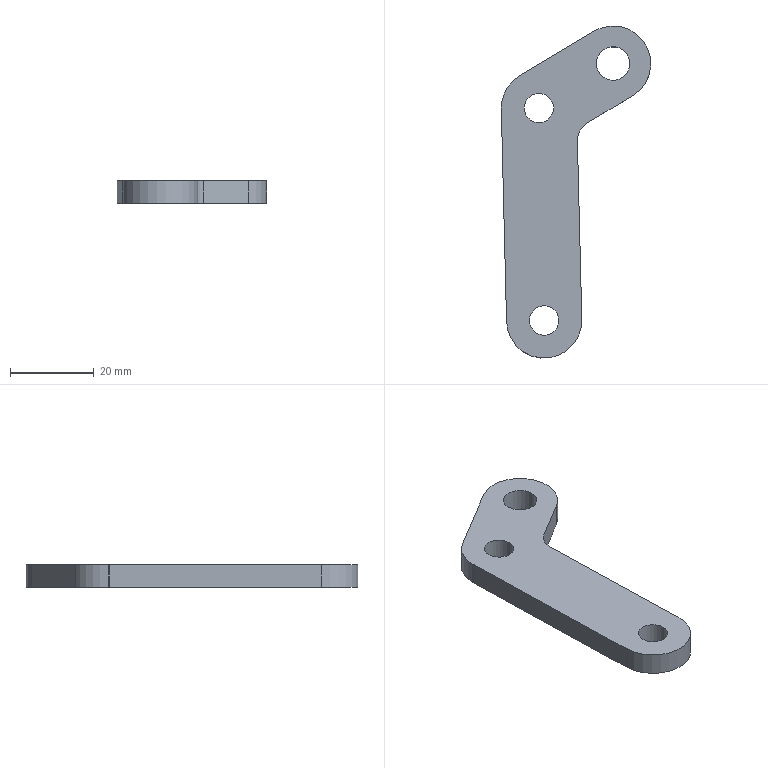Part | SolidWorks | features Extrusion 1 | 1 solid | 18 faces | box 35.738 x 79.423 x 5.4 mm | volume 7618 mm3 | cylinder 12 | plane 6 | commonest cylinder face diameters 7 x4 18 x3 8 x2 10.009 x2 17.997 x1
STEP:
#1=CARTESIAN_POINT('',(11.627,34.256,5.4));
#2=VERTEX_POINT('',#1);
#3=CARTESIAN_POINT('',(9.196,29.964,5.4));
#4=VERTEX_POINT('',#3);
#5=CARTESIAN_POINT('',(14.201,29.964,5.4));
#6=DIRECTION('',(0.,0.,1.));
#7=DIRECTION('',(1.,0.,0.));
#8=AXIS2_PLACEMENT_3D('',#5,#6,#7);
#9=CIRCLE('',#8,5.004);
#10=EDGE_CURVE('',#2,#4,#9,.T.);
#11=ORIENTED_EDGE('',*,*,#10,.T.);
#12=CARTESIAN_POINT('',(9.196,29.964,0.));
#13=VERTEX_POINT('',#12);
#14=CARTESIAN_POINT('',(9.196,29.964,5.4));
#15=DIRECTION('',(0.,0.,-1.));
#16=VECTOR('',#15,1000.);
#17=LINE('',#14,#16);
#18=EDGE_CURVE('',#4,#13,#17,.T.);
#19=ORIENTED_EDGE('',*,*,#18,.T.);
#20=CARTESIAN_POINT('',(11.627,34.256,0.));
#21=VERTEX_POINT('',#20);
#22=CARTESIAN_POINT('',(14.201,29.964,0.));
#23=DIRECTION('',(0.,0.,1.));
#24=DIRECTION('',(1.,0.,0.));
#25=AXIS2_PLACEMENT_3D('',#22,#23,#24);
#26=CIRCLE('',#25,5.004);
#27=EDGE_CURVE('',#21,#13,#26,.T.);
#28=ORIENTED_EDGE('',*,*,#27,.F.);
#29=CARTESIAN_POINT('',(11.627,34.256,5.4));
#30=DIRECTION('',(0.,0.,-1.));
#31=VECTOR('',#30,1000.);
#32=LINE('',#29,#31);
#33=EDGE_CURVE('',#2,#21,#32,.T.);
#34=ORIENTED_EDGE('',*,*,#33,.F.);
#35=EDGE_LOOP('',(#11,#19,#28,#34));
#36=FACE_OUTER_BOUND('',#35,.T.);
#37=CARTESIAN_POINT('',(14.201,29.964,5.4));
#38=DIRECTION('',(0.,0.,-1.));
#39=DIRECTION('',(-1.,0.,0.));
#40=AXIS2_PLACEMENT_3D('',#37,#38,#39);
#41=CYLINDRICAL_SURFACE('',#40,5.004);
#42=ADVANCED_FACE('',(#36),#41,.F.);
#43=CARTESIAN_POINT('',(-3.5,37.774,5.4));
#44=VERTEX_POINT('',#43);
#45=CARTESIAN_POINT('',(3.5,37.774,5.4));
#46=VERTEX_POINT('',#45);
#47=CARTESIAN_POINT('',(0.,37.774,5.4));
#48=DIRECTION('',(0.,0.,1.));
#49=DIRECTION('',(1.,0.,0.));
#50=AXIS2_PLACEMENT_3D('',#47,#48,#49);
#51=CIRCLE('',#50,3.5);
#52=EDGE_CURVE('',#44,#46,#51,.T.);
#53=ORIENTED_EDGE('',*,*,#52,.T.);
#54=CARTESIAN_POINT('',(3.5,37.774,0.));
#55=VERTEX_POINT('',#54);
#56=CARTESIAN_POINT('',(3.5,37.774,5.4));
#57=DIRECTION('',(0.,0.,-1.));
#58=VECTOR('',#57,1000.);
#59=LINE('',#56,#58);
#60=EDGE_CURVE('',#46,#55,#59,.T.);
#61=ORIENTED_EDGE('',*,*,#60,.T.);
#62=CARTESIAN_POINT('',(-3.5,37.774,0.));
#63=VERTEX_POINT('',#62);
#64=CARTESIAN_POINT('',(0.,37.774,0.));
#65=DIRECTION('',(0.,0.,1.));
#66=DIRECTION('',(1.,0.,0.));
#67=AXIS2_PLACEMENT_3D('',#64,#65,#66);
#68=CIRCLE('',#67,3.5);
#69=EDGE_CURVE('',#63,#55,#68,.T.);
#70=ORIENTED_EDGE('',*,*,#69,.F.);
#71=CARTESIAN_POINT('',(-3.5,37.774,5.4));
#72=DIRECTION('',(0.,0.,-1.));
#73=VECTOR('',#72,1000.);
#74=LINE('',#71,#73);
#75=EDGE_CURVE('',#44,#63,#74,.T.);
#76=ORIENTED_EDGE('',*,*,#75,.F.);
#77=EDGE_LOOP('',(#53,#61,#70,#76));
#78=FACE_OUTER_BOUND('',#77,.T.);
#79=CARTESIAN_POINT('',(0.,37.774,5.4));
#80=DIRECTION('',(0.,0.,-1.));
#81=DIRECTION('',(-1.,0.,0.));
#82=AXIS2_PLACEMENT_3D('',#79,#80,#81);
#83=CYLINDRICAL_SURFACE('',#82,3.5);
#84=ADVANCED_FACE('',(#78),#83,.F.);
#85=CARTESIAN_POINT('',(-2.25,-13.01,5.4));
#86=VERTEX_POINT('',#85);
#87=CARTESIAN_POINT('',(4.75,-13.01,5.4));
#88=VERTEX_POINT('',#87);
#89=CARTESIAN_POINT('',(1.25,-13.01,5.4));
#90=DIRECTION('',(0.,0.,1.));
#91=DIRECTION('',(1.,0.,0.));
#92=AXIS2_PLACEMENT_3D('',#89,#90,#91);
#93=CIRCLE('',#92,3.5);
#94=EDGE_CURVE('',#86,#88,#93,.T.);
#95=ORIENTED_EDGE('',*,*,#94,.T.);
#96=CARTESIAN_POINT('',(4.75,-13.01,0.));
#97=VERTEX_POINT('',#96);
#98=CARTESIAN_POINT('',(4.75,-13.01,5.4));
#99=DIRECTION('',(0.,0.,-1.));
#100=VECTOR('',#99,1000.);
#101=LINE('',#98,#100);
#102=EDGE_CURVE('',#88,#97,#101,.T.);
#103=ORIENTED_EDGE('',*,*,#102,.T.);
#104=CARTESIAN_POINT('',(-2.25,-13.01,0.));
#105=VERTEX_POINT('',#104);
#106=CARTESIAN_POINT('',(1.25,-13.01,0.));
#107=DIRECTION('',(0.,0.,1.));
#108=DIRECTION('',(1.,0.,0.));
#109=AXIS2_PLACEMENT_3D('',#106,#107,#108);
#110=CIRCLE('',#109,3.5);
#111=EDGE_CURVE('',#105,#97,#110,.T.);
#112=ORIENTED_EDGE('',*,*,#111,.F.);
#113=CARTESIAN_POINT('',(-2.25,-13.01,5.4));
#114=DIRECTION('',(0.,0.,-1.));
#115=VECTOR('',#114,1000.);
#116=LINE('',#113,#115);
#117=EDGE_CURVE('',#86,#105,#116,.T.);
#118=ORIENTED_EDGE('',*,*,#117,.F.);
#119=EDGE_LOOP('',(#95,#103,#112,#118));
#120=FACE_OUTER_BOUND('',#119,.T.);
#121=CARTESIAN_POINT('',(1.25,-13.01,5.4));
#122=DIRECTION('',(0.,0.,-1.));
#123=DIRECTION('',(-1.,0.,0.));
#124=AXIS2_PLACEMENT_3D('',#121,#122,#123);
#125=CYLINDRICAL_SURFACE('',#124,3.5);
#126=ADVANCED_FACE('',(#120),#125,.F.);
#127=CARTESIAN_POINT('',(13.74,48.414,5.4));
#128=VERTEX_POINT('',#127);
#129=CARTESIAN_POINT('',(21.74,48.414,5.4));
#130=VERTEX_POINT('',#129);
#131=CARTESIAN_POINT('',(17.74,48.414,5.4));
#132=DIRECTION('',(0.,0.,1.));
#133=DIRECTION('',(1.,0.,0.));
#134=AXIS2_PLACEMENT_3D('',#131,#132,#133);
#135=CIRCLE('',#134,4.);
#136=EDGE_CURVE('',#128,#130,#135,.T.);
#137=ORIENTED_EDGE('',*,*,#136,.T.);
#138=CARTESIAN_POINT('',(21.74,48.414,0.));
#139=VERTEX_POINT('',#138);
#140=CARTESIAN_POINT('',(21.74,48.414,5.4));
#141=DIRECTION('',(0.,0.,-1.));
#142=VECTOR('',#141,1000.);
#143=LINE('',#140,#142);
#144=EDGE_CURVE('',#130,#139,#143,.T.);
#145=ORIENTED_EDGE('',*,*,#144,.T.);
#146=CARTESIAN_POINT('',(13.74,48.414,0.));
#147=VERTEX_POINT('',#146);
#148=CARTESIAN_POINT('',(17.74,48.414,0.));
#149=DIRECTION('',(0.,0.,1.));
#150=DIRECTION('',(1.,0.,0.));
#151=AXIS2_PLACEMENT_3D('',#148,#149,#150);
#152=CIRCLE('',#151,4.);
#153=EDGE_CURVE('',#147,#139,#152,.T.);
#154=ORIENTED_EDGE('',*,*,#153,.F.);
#155=CARTESIAN_POINT('',(13.74,48.414,5.4));
#156=DIRECTION('',(0.,0.,-1.));
#157=VECTOR('',#156,1000.);
#158=LINE('',#155,#157);
#159=EDGE_CURVE('',#128,#147,#158,.T.);
#160=ORIENTED_EDGE('',*,*,#159,.F.);
#161=EDGE_LOOP('',(#137,#145,#154,#160));
#162=FACE_OUTER_BOUND('',#161,.T.);
#163=CARTESIAN_POINT('',(17.74,48.414,5.4));
#164=DIRECTION('',(0.,0.,-1.));
#165=DIRECTION('',(-1.,0.,0.));
#166=AXIS2_PLACEMENT_3D('',#163,#164,#165);
#167=CYLINDRICAL_SURFACE('',#166,4.);
#168=ADVANCED_FACE('',(#162),#167,.F.);
#169=CARTESIAN_POINT('',(-9.,37.774,5.4));
#170=VERTEX_POINT('',#169);
#171=CARTESIAN_POINT('',(-8.997,37.553,5.4));
#172=VERTEX_POINT('',#171);
#173=CARTESIAN_POINT('',(0.,37.774,5.4));
#174=DIRECTION('',(0.,0.,1.));
#175=DIRECTION('',(1.,0.,0.));
#176=AXIS2_PLACEMENT_3D('',#173,#174,#175);
#177=CIRCLE('',#176,9.);
#178=EDGE_CURVE('',#170,#172,#177,.T.);
#179=ORIENTED_EDGE('',*,*,#178,.F.);
#180=CARTESIAN_POINT('',(-9.,37.774,0.));
#181=VERTEX_POINT('',#180);
#182=CARTESIAN_POINT('',(-9.,37.774,5.4));
#183=DIRECTION('',(0.,0.,-1.));
#184=VECTOR('',#183,1000.);
#185=LINE('',#182,#184);
#186=EDGE_CURVE('',#170,#181,#185,.T.);
#187=ORIENTED_EDGE('',*,*,#186,.T.);
#188=CARTESIAN_POINT('',(-8.997,37.553,0.));
#189=VERTEX_POINT('',#188);
#190=CARTESIAN_POINT('',(0.,37.774,0.));
#191=DIRECTION('',(0.,0.,1.));
#192=DIRECTION('',(1.,0.,0.));
#193=AXIS2_PLACEMENT_3D('',#190,#191,#192);
#194=CIRCLE('',#193,9.);
#195=EDGE_CURVE('',#181,#189,#194,.T.);
#196=ORIENTED_EDGE('',*,*,#195,.T.);
#197=CARTESIAN_POINT('',(-8.997,37.553,5.4));
#198=DIRECTION('',(0.,0.,-1.));
#199=VECTOR('',#198,1000.);
#200=LINE('',#197,#199);
#201=EDGE_CURVE('',#172,#189,#200,.T.);
#202=ORIENTED_EDGE('',*,*,#201,.F.);
#203=EDGE_LOOP('',(#179,#187,#196,#202));
#204=FACE_OUTER_BOUND('',#203,.T.);
#205=CARTESIAN_POINT('',(0.,37.774,5.4));
#206=DIRECTION('',(0.,0.,-1.));
#207=DIRECTION('',(-1.,0.,0.));
#208=AXIS2_PLACEMENT_3D('',#205,#206,#207);
#209=CYLINDRICAL_SURFACE('',#208,9.);
#210=ADVANCED_FACE('',(#204),#209,.T.);
#211=CARTESIAN_POINT('',(22.368,40.697,0.));
#212=VERTEX_POINT('',#211);
#213=CARTESIAN_POINT('',(-12.034,20.067,0.));
#214=DIRECTION('',(-0.8576,-0.5143,0.));
#215=VECTOR('',#214,1000.);
#216=LINE('',#213,#215);
#217=EDGE_CURVE('',#212,#21,#216,.T.);
#218=ORIENTED_EDGE('',*,*,#217,.F.);
#219=CARTESIAN_POINT('',(22.368,40.697,5.4));
#220=VERTEX_POINT('',#219);
#221=CARTESIAN_POINT('',(22.368,40.697,5.4));
#222=DIRECTION('',(0.,0.,-1.));
#223=VECTOR('',#222,1000.);
#224=LINE('',#221,#223);
#225=EDGE_CURVE('',#220,#212,#224,.T.);
#226=ORIENTED_EDGE('',*,*,#225,.F.);
#227=CARTESIAN_POINT('',(-12.034,20.067,5.4));
#228=DIRECTION('',(-0.8576,-0.5143,0.));
#229=VECTOR('',#228,1000.);
#230=LINE('',#227,#229);
#231=EDGE_CURVE('',#220,#2,#230,.T.);
#232=ORIENTED_EDGE('',*,*,#231,.T.);
#233=ORIENTED_EDGE('',*,*,#33,.T.);
#234=EDGE_LOOP('',(#218,#226,#232,#233));
#235=FACE_OUTER_BOUND('',#234,.T.);
#236=CARTESIAN_POINT('',(-12.034,20.067,5.4));
#237=DIRECTION('',(0.5143,-0.8576,0.));
#238=DIRECTION('',(0.8576,0.5143,0.));
#239=AXIS2_PLACEMENT_3D('',#236,#237,#238);
#240=PLANE('',#239);
#241=ADVANCED_FACE('',(#235),#240,.T.);
#242=CARTESIAN_POINT('',(13.112,56.132,0.));
#243=VERTEX_POINT('',#242);
#244=CARTESIAN_POINT('',(17.74,48.414,0.));
#245=DIRECTION('',(0.,0.,1.));
#246=DIRECTION('',(1.,0.,0.));
#247=AXIS2_PLACEMENT_3D('',#244,#245,#246);
#248=CIRCLE('',#247,8.998);
#249=EDGE_CURVE('',#212,#243,#248,.T.);
#250=ORIENTED_EDGE('',*,*,#249,.T.);
#251=CARTESIAN_POINT('',(13.112,56.132,5.4));
#252=VERTEX_POINT('',#251);
#253=CARTESIAN_POINT('',(13.112,56.132,5.4));
#254=DIRECTION('',(0.,0.,-1.));
#255=VECTOR('',#254,1000.);
#256=LINE('',#253,#255);
#257=EDGE_CURVE('',#252,#243,#256,.T.);
#258=ORIENTED_EDGE('',*,*,#257,.F.);
#259=CARTESIAN_POINT('',(17.74,48.414,5.4));
#260=DIRECTION('',(0.,0.,1.));
#261=DIRECTION('',(1.,0.,0.));
#262=AXIS2_PLACEMENT_3D('',#259,#260,#261);
#263=CIRCLE('',#262,8.998);
#264=EDGE_CURVE('',#220,#252,#263,.T.);
#265=ORIENTED_EDGE('',*,*,#264,.F.);
#266=ORIENTED_EDGE('',*,*,#225,.T.);
#267=EDGE_LOOP('',(#250,#258,#265,#266));
#268=FACE_OUTER_BOUND('',#267,.T.);
#269=CARTESIAN_POINT('',(17.74,48.414,5.4));
#270=DIRECTION('',(0.,0.,-1.));
#271=DIRECTION('',(-1.,0.,0.));
#272=AXIS2_PLACEMENT_3D('',#269,#270,#271);
#273=CYLINDRICAL_SURFACE('',#272,8.998);
#274=ADVANCED_FACE('',(#268),#273,.T.);
#275=CARTESIAN_POINT('',(-4.629,45.493,0.));
#276=VERTEX_POINT('',#275);
#277=CARTESIAN_POINT('',(-21.289,35.502,0.));
#278=DIRECTION('',(0.8576,0.5143,0.));
#279=VECTOR('',#278,1000.);
#280=LINE('',#277,#279);
#281=EDGE_CURVE('',#276,#243,#280,.T.);
#282=ORIENTED_EDGE('',*,*,#281,.F.);
#283=CARTESIAN_POINT('',(-4.629,45.493,5.4));
#284=VERTEX_POINT('',#283);
#285=CARTESIAN_POINT('',(-4.629,45.493,5.4));
#286=DIRECTION('',(0.,0.,-1.));
#287=VECTOR('',#286,1000.);
#288=LINE('',#285,#287);
#289=EDGE_CURVE('',#284,#276,#288,.T.);
#290=ORIENTED_EDGE('',*,*,#289,.F.);
#291=CARTESIAN_POINT('',(-21.289,35.502,5.4));
#292=DIRECTION('',(0.8576,0.5143,0.));
#293=VECTOR('',#292,1000.);
#294=LINE('',#291,#293);
#295=EDGE_CURVE('',#284,#252,#294,.T.);
#296=ORIENTED_EDGE('',*,*,#295,.T.);
#297=ORIENTED_EDGE('',*,*,#257,.T.);
#298=EDGE_LOOP('',(#282,#290,#296,#297));
#299=FACE_OUTER_BOUND('',#298,.T.);
#300=CARTESIAN_POINT('',(-21.289,35.502,5.4));
#301=DIRECTION('',(-0.5143,0.8576,0.));
#302=DIRECTION('',(-0.8576,-0.5143,0.));
#303=AXIS2_PLACEMENT_3D('',#300,#301,#302);
#304=PLANE('',#303);
#305=ADVANCED_FACE('',(#299),#304,.T.);
#306=ORIENTED_EDGE('',*,*,#186,.F.);
#307=CARTESIAN_POINT('',(0.,37.774,5.4));
#308=DIRECTION('',(0.,0.,1.));
#309=DIRECTION('',(1.,0.,0.));
#310=AXIS2_PLACEMENT_3D('',#307,#308,#309);
#311=CIRCLE('',#310,9.);
#312=EDGE_CURVE('',#284,#170,#311,.T.);
#313=ORIENTED_EDGE('',*,*,#312,.F.);
#314=ORIENTED_EDGE('',*,*,#289,.T.);
#315=CARTESIAN_POINT('',(0.,37.774,0.));
#316=DIRECTION('',(0.,0.,1.));
#317=DIRECTION('',(1.,0.,0.));
#318=AXIS2_PLACEMENT_3D('',#315,#316,#317);
#319=CIRCLE('',#318,9.);
#320=EDGE_CURVE('',#276,#181,#319,.T.);
#321=ORIENTED_EDGE('',*,*,#320,.T.);
#322=EDGE_LOOP('',(#306,#313,#314,#321));
#323=FACE_OUTER_BOUND('',#322,.T.);
#324=CARTESIAN_POINT('',(0.,37.774,5.4));
#325=DIRECTION('',(0.,0.,-1.));
#326=DIRECTION('',(-1.,0.,0.));
#327=AXIS2_PLACEMENT_3D('',#324,#325,#326);
#328=CYLINDRICAL_SURFACE('',#327,9.);
#329=ADVANCED_FACE('',(#323),#328,.T.);
#330=CARTESIAN_POINT('',(-7.747,-13.232,0.));
#331=VERTEX_POINT('',#330);
#332=CARTESIAN_POINT('',(-8.068,-0.1986,0.));
#333=DIRECTION('',(0.02461,-0.9997,0.));
#334=VECTOR('',#333,1000.);
#335=LINE('',#332,#334);
#336=EDGE_CURVE('',#189,#331,#335,.T.);
#337=ORIENTED_EDGE('',*,*,#336,.T.);
#338=CARTESIAN_POINT('',(-7.747,-13.232,5.4));
#339=VERTEX_POINT('',#338);
#340=CARTESIAN_POINT('',(-7.747,-13.232,5.4));
#341=DIRECTION('',(0.,0.,-1.));
#342=VECTOR('',#341,1000.);
#343=LINE('',#340,#342);
#344=EDGE_CURVE('',#339,#331,#343,.T.);
#345=ORIENTED_EDGE('',*,*,#344,.F.);
#346=CARTESIAN_POINT('',(-8.068,-0.1986,5.4));
#347=DIRECTION('',(0.02461,-0.9997,0.));
#348=VECTOR('',#347,1000.);
#349=LINE('',#346,#348);
#350=EDGE_CURVE('',#172,#339,#349,.T.);
#351=ORIENTED_EDGE('',*,*,#350,.F.);
#352=ORIENTED_EDGE('',*,*,#201,.T.);
#353=EDGE_LOOP('',(#337,#345,#351,#352));
#354=FACE_OUTER_BOUND('',#353,.T.);
#355=CARTESIAN_POINT('',(-8.068,-0.1986,5.4));
#356=DIRECTION('',(0.9997,0.02461,0.));
#357=DIRECTION('',(-0.02461,0.9997,0.));
#358=AXIS2_PLACEMENT_3D('',#355,#356,#357);
#359=PLANE('',#358);
#360=ADVANCED_FACE('',(#354),#359,.F.);
#361=CARTESIAN_POINT('',(10.247,-12.789,0.));
#362=VERTEX_POINT('',#361);
#363=CARTESIAN_POINT('',(1.25,-13.01,0.));
#364=DIRECTION('',(0.,0.,1.));
#365=DIRECTION('',(1.,0.,0.));
#366=AXIS2_PLACEMENT_3D('',#363,#364,#365);
#367=CIRCLE('',#366,9.);
#368=EDGE_CURVE('',#331,#362,#367,.T.);
#369=ORIENTED_EDGE('',*,*,#368,.T.);
#370=CARTESIAN_POINT('',(10.247,-12.789,5.4));
#371=VERTEX_POINT('',#370);
#372=CARTESIAN_POINT('',(10.247,-12.789,5.4));
#373=DIRECTION('',(0.,0.,-1.));
#374=VECTOR('',#373,1000.);
#375=LINE('',#372,#374);
#376=EDGE_CURVE('',#371,#362,#375,.T.);
#377=ORIENTED_EDGE('',*,*,#376,.F.);
#378=CARTESIAN_POINT('',(1.25,-13.01,5.4));
#379=DIRECTION('',(0.,0.,1.));
#380=DIRECTION('',(1.,0.,0.));
#381=AXIS2_PLACEMENT_3D('',#378,#379,#380);
#382=CIRCLE('',#381,9.);
#383=EDGE_CURVE('',#339,#371,#382,.T.);
#384=ORIENTED_EDGE('',*,*,#383,.F.);
#385=ORIENTED_EDGE('',*,*,#344,.T.);
#386=EDGE_LOOP('',(#369,#377,#384,#385));
#387=FACE_OUTER_BOUND('',#386,.T.);
#388=CARTESIAN_POINT('',(1.25,-13.01,5.4));
#389=DIRECTION('',(0.,0.,-1.));
#390=DIRECTION('',(-1.,0.,0.));
#391=AXIS2_PLACEMENT_3D('',#388,#389,#390);
#392=CYLINDRICAL_SURFACE('',#391,9.);
#393=ADVANCED_FACE('',(#387),#392,.T.);
#394=CARTESIAN_POINT('',(9.198,29.841,0.));
#395=VERTEX_POINT('',#394);
#396=CARTESIAN_POINT('',(9.926,0.2443,0.));
#397=DIRECTION('',(0.02461,-0.9997,0.));
#398=VECTOR('',#397,1000.);
#399=LINE('',#396,#398);
#400=EDGE_CURVE('',#395,#362,#399,.T.);
#401=ORIENTED_EDGE('',*,*,#400,.F.);
#402=CARTESIAN_POINT('',(9.198,29.841,5.4));
#403=VERTEX_POINT('',#402);
#404=CARTESIAN_POINT('',(9.198,29.841,5.4));
#405=DIRECTION('',(0.,0.,-1.));
#406=VECTOR('',#405,1000.);
#407=LINE('',#404,#406);
#408=EDGE_CURVE('',#403,#395,#407,.T.);
#409=ORIENTED_EDGE('',*,*,#408,.F.);
#410=CARTESIAN_POINT('',(9.926,0.2443,5.4));
#411=DIRECTION('',(0.02461,-0.9997,0.));
#412=VECTOR('',#411,1000.);
#413=LINE('',#410,#412);
#414=EDGE_CURVE('',#403,#371,#413,.T.);
#415=ORIENTED_EDGE('',*,*,#414,.T.);
#416=ORIENTED_EDGE('',*,*,#376,.T.);
#417=EDGE_LOOP('',(#401,#409,#415,#416));
#418=FACE_OUTER_BOUND('',#417,.T.);
#419=CARTESIAN_POINT('',(9.926,0.2443,5.4));
#420=DIRECTION('',(0.9997,0.02461,0.));
#421=DIRECTION('',(-0.02461,0.9997,0.));
#422=AXIS2_PLACEMENT_3D('',#419,#420,#421);
#423=PLANE('',#422);
#424=ADVANCED_FACE('',(#418),#423,.T.);
#425=ORIENTED_EDGE('',*,*,#144,.F.);
#426=CARTESIAN_POINT('',(17.74,48.414,5.4));
#427=DIRECTION('',(0.,0.,1.));
#428=DIRECTION('',(1.,0.,0.));
#429=AXIS2_PLACEMENT_3D('',#426,#427,#428);
#430=CIRCLE('',#429,4.);
#431=EDGE_CURVE('',#130,#128,#430,.T.);
#432=ORIENTED_EDGE('',*,*,#431,.T.);
#433=ORIENTED_EDGE('',*,*,#159,.T.);
#434=CARTESIAN_POINT('',(17.74,48.414,0.));
#435=DIRECTION('',(0.,0.,1.));
#436=DIRECTION('',(1.,0.,0.));
#437=AXIS2_PLACEMENT_3D('',#434,#435,#436);
#438=CIRCLE('',#437,4.);
#439=EDGE_CURVE('',#139,#147,#438,.T.);
#440=ORIENTED_EDGE('',*,*,#439,.F.);
#441=EDGE_LOOP('',(#425,#432,#433,#440));
#442=FACE_OUTER_BOUND('',#441,.T.);
#443=CARTESIAN_POINT('',(17.74,48.414,5.4));
#444=DIRECTION('',(0.,0.,-1.));
#445=DIRECTION('',(-1.,0.,0.));
#446=AXIS2_PLACEMENT_3D('',#443,#444,#445);
#447=CYLINDRICAL_SURFACE('',#446,4.);
#448=ADVANCED_FACE('',(#442),#447,.F.);
#449=ORIENTED_EDGE('',*,*,#102,.F.);
#450=CARTESIAN_POINT('',(1.25,-13.01,5.4));
#451=DIRECTION('',(0.,0.,1.));
#452=DIRECTION('',(1.,0.,0.));
#453=AXIS2_PLACEMENT_3D('',#450,#451,#452);
#454=CIRCLE('',#453,3.5);
#455=EDGE_CURVE('',#88,#86,#454,.T.);
#456=ORIENTED_EDGE('',*,*,#455,.T.);
#457=ORIENTED_EDGE('',*,*,#117,.T.);
#458=CARTESIAN_POINT('',(1.25,-13.01,0.));
#459=DIRECTION('',(0.,0.,1.));
#460=DIRECTION('',(1.,0.,0.));
#461=AXIS2_PLACEMENT_3D('',#458,#459,#460);
#462=CIRCLE('',#461,3.5);
#463=EDGE_CURVE('',#97,#105,#462,.T.);
#464=ORIENTED_EDGE('',*,*,#463,.F.);
#465=EDGE_LOOP('',(#449,#456,#457,#464));
#466=FACE_OUTER_BOUND('',#465,.T.);
#467=CARTESIAN_POINT('',(1.25,-13.01,5.4));
#468=DIRECTION('',(0.,0.,-1.));
#469=DIRECTION('',(-1.,0.,0.));
#470=AXIS2_PLACEMENT_3D('',#467,#468,#469);
#471=CYLINDRICAL_SURFACE('',#470,3.5);
#472=ADVANCED_FACE('',(#466),#471,.F.);
#473=ORIENTED_EDGE('',*,*,#60,.F.);
#474=CARTESIAN_POINT('',(0.,37.774,5.4));
#475=DIRECTION('',(0.,0.,1.));
#476=DIRECTION('',(1.,0.,0.));
#477=AXIS2_PLACEMENT_3D('',#474,#475,#476);
#478=CIRCLE('',#477,3.5);
#479=EDGE_CURVE('',#46,#44,#478,.T.);
#480=ORIENTED_EDGE('',*,*,#479,.T.);
#481=ORIENTED_EDGE('',*,*,#75,.T.);
#482=CARTESIAN_POINT('',(0.,37.774,0.));
#483=DIRECTION('',(0.,0.,1.));
#484=DIRECTION('',(1.,0.,0.));
#485=AXIS2_PLACEMENT_3D('',#482,#483,#484);
#486=CIRCLE('',#485,3.5);
#487=EDGE_CURVE('',#55,#63,#486,.T.);
#488=ORIENTED_EDGE('',*,*,#487,.F.);
#489=EDGE_LOOP('',(#473,#480,#481,#488));
#490=FACE_OUTER_BOUND('',#489,.T.);
#491=CARTESIAN_POINT('',(0.,37.774,5.4));
#492=DIRECTION('',(0.,0.,-1.));
#493=DIRECTION('',(-1.,0.,0.));
#494=AXIS2_PLACEMENT_3D('',#491,#492,#493);
#495=CYLINDRICAL_SURFACE('',#494,3.5);
#496=ADVANCED_FACE('',(#490),#495,.F.);
#497=ORIENTED_EDGE('',*,*,#18,.F.);
#498=CARTESIAN_POINT('',(14.201,29.964,5.4));
#499=DIRECTION('',(0.,0.,1.));
#500=DIRECTION('',(1.,0.,0.));
#501=AXIS2_PLACEMENT_3D('',#498,#499,#500);
#502=CIRCLE('',#501,5.004);
#503=EDGE_CURVE('',#4,#403,#502,.T.);
#504=ORIENTED_EDGE('',*,*,#503,.T.);
#505=ORIENTED_EDGE('',*,*,#408,.T.);
#506=CARTESIAN_POINT('',(14.201,29.964,0.));
#507=DIRECTION('',(0.,0.,1.));
#508=DIRECTION('',(1.,0.,0.));
#509=AXIS2_PLACEMENT_3D('',#506,#507,#508);
#510=CIRCLE('',#509,5.004);
#511=EDGE_CURVE('',#13,#395,#510,.T.);
#512=ORIENTED_EDGE('',*,*,#511,.F.);
#513=EDGE_LOOP('',(#497,#504,#505,#512));
#514=FACE_OUTER_BOUND('',#513,.T.);
#515=CARTESIAN_POINT('',(14.201,29.964,5.4));
#516=DIRECTION('',(0.,0.,-1.));
#517=DIRECTION('',(-1.,0.,0.));
#518=AXIS2_PLACEMENT_3D('',#515,#516,#517);
#519=CYLINDRICAL_SURFACE('',#518,5.004);
#520=ADVANCED_FACE('',(#514),#519,.F.);
#521=ORIENTED_EDGE('',*,*,#52,.F.);
#522=ORIENTED_EDGE('',*,*,#479,.F.);
#523=EDGE_LOOP('',(#521,#522));
#524=FACE_BOUND('',#523,.T.);
#525=ORIENTED_EDGE('',*,*,#94,.F.);
#526=ORIENTED_EDGE('',*,*,#455,.F.);
#527=EDGE_LOOP('',(#525,#526));
#528=FACE_BOUND('',#527,.T.);
#529=ORIENTED_EDGE('',*,*,#136,.F.);
#530=ORIENTED_EDGE('',*,*,#431,.F.);
#531=EDGE_LOOP('',(#529,#530));
#532=FACE_BOUND('',#531,.T.);
#533=ORIENTED_EDGE('',*,*,#231,.F.);
#534=ORIENTED_EDGE('',*,*,#264,.T.);
#535=ORIENTED_EDGE('',*,*,#295,.F.);
#536=ORIENTED_EDGE('',*,*,#312,.T.);
#537=ORIENTED_EDGE('',*,*,#178,.T.);
#538=ORIENTED_EDGE('',*,*,#350,.T.);
#539=ORIENTED_EDGE('',*,*,#383,.T.);
#540=ORIENTED_EDGE('',*,*,#414,.F.);
#541=ORIENTED_EDGE('',*,*,#503,.F.);
#542=ORIENTED_EDGE('',*,*,#10,.F.);
#543=EDGE_LOOP('',(#533,#534,#535,#536,#537,#538,#539,#540,#541,#542));
#544=FACE_OUTER_BOUND('',#543,.T.);
#545=CARTESIAN_POINT('',(0.,0.,5.4));
#546=DIRECTION('',(0.,0.,1.));
#547=DIRECTION('',(1.,0.,0.));
#548=AXIS2_PLACEMENT_3D('',#545,#546,#547);
#549=PLANE('',#548);
#550=ADVANCED_FACE('',(#524,#528,#532,#544),#549,.T.);
#551=ORIENTED_EDGE('',*,*,#69,.T.);
#552=ORIENTED_EDGE('',*,*,#487,.T.);
#553=EDGE_LOOP('',(#551,#552));
#554=FACE_BOUND('',#553,.T.);
#555=ORIENTED_EDGE('',*,*,#111,.T.);
#556=ORIENTED_EDGE('',*,*,#463,.T.);
#557=EDGE_LOOP('',(#555,#556));
#558=FACE_BOUND('',#557,.T.);
#559=ORIENTED_EDGE('',*,*,#153,.T.);
#560=ORIENTED_EDGE('',*,*,#439,.T.);
#561=EDGE_LOOP('',(#559,#560));
#562=FACE_BOUND('',#561,.T.);
#563=ORIENTED_EDGE('',*,*,#217,.T.);
#564=ORIENTED_EDGE('',*,*,#27,.T.);
#565=ORIENTED_EDGE('',*,*,#511,.T.);
#566=ORIENTED_EDGE('',*,*,#400,.T.);
#567=ORIENTED_EDGE('',*,*,#368,.F.);
#568=ORIENTED_EDGE('',*,*,#336,.F.);
#569=ORIENTED_EDGE('',*,*,#195,.F.);
#570=ORIENTED_EDGE('',*,*,#320,.F.);
#571=ORIENTED_EDGE('',*,*,#281,.T.);
#572=ORIENTED_EDGE('',*,*,#249,.F.);
#573=EDGE_LOOP('',(#563,#564,#565,#566,#567,#568,#569,#570,#571,#572));
#574=FACE_OUTER_BOUND('',#573,.T.);
#575=CARTESIAN_POINT('',(0.,0.,0.));
#576=DIRECTION('',(0.,0.,1.));
#577=DIRECTION('',(1.,0.,0.));
#578=AXIS2_PLACEMENT_3D('',#575,#576,#577);
#579=PLANE('',#578);
#580=ADVANCED_FACE('',(#554,#558,#562,#574),#579,.F.);
#581=CLOSED_SHELL('',(#42,#84,#126,#168,#210,#241,#274,#305,#329,#360,#393,#424,#448,#472,#496,#520,#550,#580));
#582=MANIFOLD_SOLID_BREP('',#581);
#583=CARTESIAN_POINT('',(0.,0.,0.));
#584=DIRECTION('',(0.,0.,1.));
#585=DIRECTION('',(1.,0.,0.));
#586=AXIS2_PLACEMENT_3D('',#583,#584,#585);
#587=(LENGTH_UNIT()NAMED_UNIT(*)SI_UNIT(.MILLI.,.METRE.));
#588=UNCERTAINTY_MEASURE_WITH_UNIT(LENGTH_MEASURE(0.00001),#587,'','');
#589=(NAMED_UNIT(*)PLANE_ANGLE_UNIT()SI_UNIT($,.RADIAN.));
#590=(NAMED_UNIT(*)SI_UNIT($,.STERADIAN.)SOLID_ANGLE_UNIT());
#591=(GEOMETRIC_REPRESENTATION_CONTEXT(3)GLOBAL_UNCERTAINTY_ASSIGNED_CONTEXT((#588))GLOBAL_UNIT_ASSIGNED_CONTEXT((#587,#589,#590))REPRESENTATION_CONTEXT('',''));
#592=ADVANCED_BREP_SHAPE_REPRESENTATION('',(#582,#586),#591);